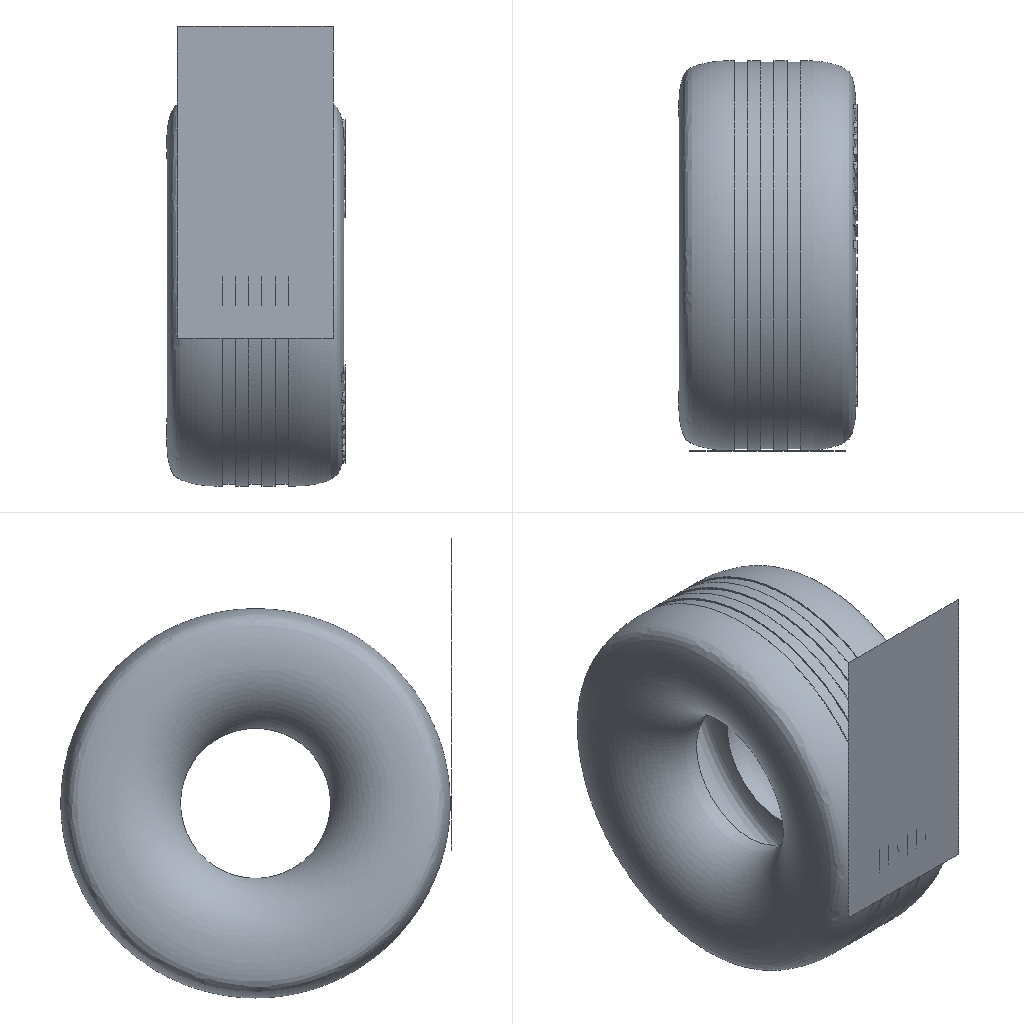Simulation study | abaqus
Set-up summary:
category,name,step,type,value,unit,region
solver,abaqus
solver,version,,,Abaqus/Explicit 2020
units,not stated in the deck,,not stated
analysis,deck,,transient,transient
load_step,Step-1,Step-1,transient
load_step,requested,,,1
mesh,nodes,,,158622
mesh,elements,,,81941
element_type,S4,,shell,5000
element_type,C3D10M,,solid,76941
load,load commands in deck,,count,3
bc,support commands in deck,,count,6
material,STEEL,,in results
material,XIANGJIAO,,in results
check,setup vs results,,match,"per instance, exact: element labels, types and connectivity; labels of the nodes the elements use; coordinates not compared"
Abaqus input file, long lists of numbers shortened:
*Heading
** Job name: Job-2 Model name: Model-2
** Generated by: Abaqus/CAE 2020
*Preprint, echo=NO, model=NO, history=NO, contact=NO
**
** PARTS
**
*Part, name=another-2
*Node
      1,       -273.5,           0.,         465.
      2,       -273.5,           0.,         485.
** (153469 more lines like these left out)
*Element, type=C3D10M
    1,  25421,    405,  19679,    406,  25558,  25557,  25556,  25560,  25559,  25561
    2,  25421,    233,    406,    220,  25563,  25562,  25560,  25565,  25564,  25566
** (76939 more lines like these left out)
*Nset, nset=Set-3, generate
      1,  153471,       1
*Elset, elset=Set-3, generate
     1,  76941,      1
** Section: xiangjiao
*Solid Section, elset=Set-3, material=xiangjiao
,
*End Part
**
*Part, name=road
*Node
      1,         290.,         915.,           0.
      2,         280.,         915.,           0.
** (5149 more lines like these left out)
*Element, type=S4
   1,    1,    2,   53,   52
   2,    2,    3,   54,   53
** (4998 more lines like these left out)
*Nset, nset=Set-1, generate
    1,  5151,     1
*Elset, elset=Set-1, generate
    1,  5000,     1
** Section: Section-1
*Shell Section, elset=Set-1, material=steel
10., 5
*End Part
**
**
** ASSEMBLY
**
*Assembly, name=Assembly
**
*Instance, name=road-1, part=road
        -40.,       -626.5,         -65.
        -40.,       -626.5,         -65., -39.,       -626.5,         -65., 90.
*End Instance
**
*Instance, name=another-2-1, part=another-2
*End Instance
**
*Node
      1,           0.,           0.,           0.
*Node
      2,         250.,       -626.5,         350.
*Nset, nset=Set-2, instance=road-1, generate
    1,  5151,     1
*Elset, elset=Set-2, instance=road-1, generate
    1,  5000,     1
*Nset, nset=Set-3
 1,
*Nset, nset=Set-5
 1,
*Nset, nset=Set-6
 1,
*Nset, nset=Set-7
 1,
*Nset, nset=Set-8
 1,
*Nset, nset=Set-9
 1,
*Nset, nset=Set-10
 1,
*Nset, nset=Set-13
 2,
*Nset, nset=Set-14
 2,
*Nset, nset=Set-15
 2,
*Nset, nset=Set-16
 1,
*Nset, nset=b_Set-11, instance=road-1, generate
    1,  5151,     1
*Elset, elset=b_Set-11, instance=road-1, generate
    1,  5000,     1
*Nset, nset=m_Set-1
 1,
*Nset, nset=_PickedSet569, internal
 2,
*Elset, elset=_m_Surf-6_S3, internal, instance=another-2-1
     2,     4,    11,    12,    21,    25,    27,    28,    33,    35,    36,    39,    44,    46,    52,    57
    63,    64,    68,    74,    80,    82,    95,   101,   110,   111,   113,   115,   117,   119,   125,   132
** (1293 more lines like these left out)
*Elset, elset=_m_Surf-6_S2, internal, instance=another-2-1
    13,    17,    24,    48,    76,    90,    91,   114,   130,   157,   162,   167,   189,   201,   203,   218
   219,   221,   223,   227,   236,   240,   244,   250,   253,   258,   260,   262,   264,   283,   286,   301
** (696 more lines like these left out)
*Elset, elset=_m_Surf-6_S4, internal, instance=another-2-1
    13,    17,    24,    72,    76,    90,    91,   127,   131,   138,   143,   144,   148,   149,   177,   182
   187,   200,   205,   209,   228,   229,   235,   239,   241,   249,   270,   287,   289,   315,   317,   340
** (553 more lines like these left out)
*Elset, elset=_m_Surf-6_S1, internal, instance=another-2-1
    77,    81,   102,   137,   142,   145,   147,   152,   163,   171,   176,   179,   183,   184,   188,   191
   194,   196,   199,   204,   213,   222,   254,   261,   292,   295,   298,   306,   312,   325,   327,   331
** (628 more lines like these left out)
*Surface, type=ELEMENT, name=m_Surf-6
_m_Surf-6_S3, S3
_m_Surf-6_S2, S2
_m_Surf-6_S4, S4
_m_Surf-6_S1, S1
*Elset, elset=_s_Surf-2_SNEG, internal, instance=road-1, generate
    1,  5000,     1
*Surface, type=ELEMENT, name=s_Surf-2
_s_Surf-2_SNEG, SNEG
*Elset, elset=_s_Surf-7_S2, internal, instance=another-2-1
   283,   778,   861,   891,  1202,  2571,  3390,  3572,  3582, 12767, 13246, 13428, 13452, 13654, 13655, 13845
 14168, 14374, 14473, 14524, 14556, 14585, 14654, 14658, 14901, 15060, 15256, 16243, 16332, 16818, 16869, 16954
** (48 more lines like these left out)
*Elset, elset=_s_Surf-7_S4, internal, instance=another-2-1
   534,  2030,  2716,  2979,  3068,  3096,  3405,  4405,  4516,  4563,  4617,  4650,  4711,  4880,  4964,  5366
  6105,  6179,  6937,  7172,  7302,  7446,  7558,  7648,  7711,  8438,  8761,  8846,  8929,  9299,  9464,  9589
** (42 more lines like these left out)
*Elset, elset=_s_Surf-7_S1, internal, instance=another-2-1
   147,  3780,  8101, 13221, 13303, 13883, 13888, 14132, 14412, 14921, 15604, 16206, 16210, 16278, 16845, 16964
 16975, 16991, 17238, 17275, 17350, 17860, 18733, 18770, 19022, 19134, 19143, 19535, 19597, 19622, 19631, 20059
** (38 more lines like these left out)
*Elset, elset=_s_Surf-7_S3, internal, instance=another-2-1
  3700,  8895,  9283,  9724, 10450, 12013, 12635, 12756, 12771, 12774, 12786, 12808, 12819, 12862, 12867, 12873
 12899, 12956, 12958, 13048, 13059, 13120, 13146, 13269, 13272, 13330, 13347, 13350, 13362, 13403, 13407, 13453
** (250 more lines like these left out)
*Surface, type=ELEMENT, name=s_Surf-7
_s_Surf-7_S2, S2
_s_Surf-7_S4, S4
_s_Surf-7_S1, S1
_s_Surf-7_S3, S3
*Elset, elset=_s_Surf-8_S1, internal, instance=another-2-1
   183,   602,   880,  1021,  1075,  1262,  1336,  1680,  1805,  1959,  1971,  2449,  2454,  2666,  2884,  2893
  3035,  3055,  3091,  3385,  3681,  3705,  3766,  3799,  3957,  4087,  4195,  4225,  4789,  4989,  5059,  5207
** (25 more lines like these left out)
*Elset, elset=_s_Surf-8_S2, internal, instance=another-2-1
   223,   310,   402,   647,   824,  2323,  2381,  2720,  3745,  3875,  4029,  4113,  4167,  5371,  5416,  5515
  6377,  7873,  8407,  8416,  8421,  8429,  8435,  8436,  8441,  8454,  8457,  8472,  8477,  8489,  8491,  8496
** (27 more lines like these left out)
*Elset, elset=_s_Surf-8_S4, internal, instance=another-2-1
   182,   351,   461,   471,   592,   640,   648,   654,   798,   810,   834,   986,  1061,  1207,  1269,  1474
  1634,  1707,  1708,  1927,  1976,  1986,  2055,  2143,  2235,  2291,  2459,  2586,  2791,  2992,  3083,  3110
** (28 more lines like these left out)
*Elset, elset=_s_Surf-8_S3, internal, instance=another-2-1
   132,   133,   134,   140,   146,   159,   160,   178,   180,   195,   202,   210,   212,   214,   216,   226
   230,   231,   247,   255,   256,   257,   267,   268,   271,   274,   281,   284,   302,   303,   304,   309
** (366 more lines like these left out)
*Surface, type=ELEMENT, name=s_Surf-8
_s_Surf-8_S1, S1
_s_Surf-8_S2, S2
_s_Surf-8_S4, S4
_s_Surf-8_S3, S3
*Elset, elset=_s_Surf-9_S2, internal, instance=another-2-1
   283,   778,   861,   891,  1202,  2571,  3390,  3572,  3582, 12767, 13246, 13428, 13452, 13654, 13655, 13845
 14168, 14374, 14473, 14524, 14556, 14585, 14654, 14658, 14901, 15060, 15256, 16243, 16332, 16818, 16869, 16954
** (48 more lines like these left out)
*Elset, elset=_s_Surf-9_S4, internal, instance=another-2-1
   534,  2030,  2716,  2979,  3068,  3096,  3405,  4405,  4516,  4563,  4617,  4650,  4711,  4880,  4964,  5366
  6105,  6179,  6937,  7172,  7302,  7446,  7558,  7648,  7711,  8438,  8761,  8846,  8929,  9299,  9464,  9589
** (42 more lines like these left out)
*Elset, elset=_s_Surf-9_S1, internal, instance=another-2-1
   147,  3780,  8101, 13221, 13303, 13883, 13888, 14132, 14412, 14921, 15604, 16206, 16210, 16278, 16845, 16964
 16975, 16991, 17238, 17275, 17350, 17860, 18733, 18770, 19022, 19134, 19143, 19535, 19597, 19622, 19631, 20059
** (38 more lines like these left out)
*Elset, elset=_s_Surf-9_S3, internal, instance=another-2-1
  3700,  8895,  9283,  9724, 10450, 12013, 12635, 12756, 12771, 12774, 12786, 12808, 12819, 12862, 12867, 12873
 12899, 12956, 12958, 13048, 13059, 13120, 13146, 13269, 13272, 13330, 13347, 13350, 13362, 13403, 13407, 13453
** (250 more lines like these left out)
*Surface, type=ELEMENT, name=s_Surf-9
_s_Surf-9_S2, S2
_s_Surf-9_S4, S4
_s_Surf-9_S1, S1
_s_Surf-9_S3, S3
*Elset, elset=_s_Surf-10_S3, internal, instance=another-2-1
    46,    52,    57,    63,    64,    68,   125,   156,   215,   332,   408,   440,   445,   490,   491,   626
   652,   655,   664,   684,   739,   787,   811,   876,   944,  1031,  1039,  1057,  1183,  1197,  1496,  1561
** (90 more lines like these left out)
*Elset, elset=_s_Surf-10_S2, internal, instance=another-2-1
    48,   130,   157,   162,   167,   189,   201,   203,   218,   219,   221,   227,   236,   240,   244,   250
   253,   258,   262,   264,   286,   301,   305,   307,   311,   314,   321,   323,   330,   334,   335,   337
** (416 more lines like these left out)
*Elset, elset=_s_Surf-10_S4, internal, instance=another-2-1
    72,   127,   131,   138,   143,   144,   148,   149,   177,   187,   200,   205,   209,   228,   229,   235
   239,   241,   249,   270,   287,   289,   315,   317,   348,   366,   376,   387,   420,   435,   441,   459
** (273 more lines like these left out)
*Elset, elset=_s_Surf-10_S1, internal, instance=another-2-1
    81,   137,   142,   145,   152,   163,   171,   176,   179,   184,   188,   191,   194,   196,   199,   204
   213,   222,   254,   261,   292,   295,   298,   306,   312,   325,   327,   331,   339,   341,   353,   364
** (368 more lines like these left out)
*Surface, type=ELEMENT, name=s_Surf-10
_s_Surf-10_S3, S3
_s_Surf-10_S2, S2
_s_Surf-10_S4, S4
_s_Surf-10_S1, S1
*Elset, elset=_s_Surf-11_S3, internal, instance=another-2-1
    46,    52,    57,    63,    64,    68,   125,   156,   215,   332,   408,   440,   445,   490,   491,   626
   652,   655,   664,   684,   739,   787,   811,   876,   944,  1031,  1039,  1057,  1183,  1197,  1496,  1561
** (90 more lines like these left out)
*Elset, elset=_s_Surf-11_S2, internal, instance=another-2-1
    48,   130,   157,   162,   167,   189,   201,   203,   218,   219,   221,   227,   236,   240,   244,   250
   253,   258,   262,   264,   286,   301,   305,   307,   311,   314,   321,   323,   330,   334,   335,   337
** (416 more lines like these left out)
*Elset, elset=_s_Surf-11_S4, internal, instance=another-2-1
    72,   127,   131,   138,   143,   144,   148,   149,   177,   187,   200,   205,   209,   228,   229,   235
   239,   241,   249,   270,   287,   289,   315,   317,   348,   366,   376,   387,   420,   435,   441,   459
** (273 more lines like these left out)
*Elset, elset=_s_Surf-11_S1, internal, instance=another-2-1
    81,   137,   142,   145,   152,   163,   171,   176,   179,   184,   188,   191,   194,   196,   199,   204
   213,   222,   254,   261,   292,   295,   298,   306,   312,   325,   327,   331,   339,   341,   353,   364
** (368 more lines like these left out)
*Surface, type=ELEMENT, name=s_Surf-11
_s_Surf-11_S3, S3
_s_Surf-11_S2, S2
_s_Surf-11_S4, S4
_s_Surf-11_S1, S1
*Elset, elset=_s_Surf-12_S1, internal, instance=another-2-1
  8410,  8474,  8493,  8543,  8557,  8567,  8624,  8628,  8662,  8678,  8684,  8712,  8715,  8722,  8723,  8732
  8738,  8745,  8758,  8760,  8762,  8764,  8772,  8778,  8783,  8789,  8792,  8793,  8863,  8890,  8898,  8913
** (11 more lines like these left out)
*Elset, elset=_s_Surf-12_S2, internal, instance=another-2-1
  3875,  8407,  8421,  8429,  8435,  8436,  8441,  8454,  8457,  8472,  8477,  8489,  8491,  8496,  8500,  8509
  8521,  8522,  8528,  8562,  8563,  8574,  8581,  8593,  8639,  8664,  8669,  8677,  8692,  8699,  8703,  8727
** (13 more lines like these left out)
*Elset, elset=_s_Surf-12_S4, internal, instance=another-2-1
  8443,  8448,  8461,  8490,  8510,  8513,  8538,  8572,  8582,  8584,  8595,  8603,  8616,  8623,  8629,  8634
  8641,  8649,  8655,  8672,  8690,  8701,  8710,  8731,  8750,  8787,  8825,  8840,  8861,  8880,  8966,  8987
** (7 more lines like these left out)
*Elset, elset=_s_Surf-12_S3, internal, instance=another-2-1
  8402,  8517,  8597,  8807,  8869,  8924,  9017, 12719, 13188, 13313, 14043, 17672, 20150, 22182, 24037, 25288
 25334, 25508, 25831, 26030, 27076, 27959, 28127, 28290, 33836, 34574, 71737
*Surface, type=ELEMENT, name=s_Surf-12
_s_Surf-12_S1, S1
_s_Surf-12_S2, S2
_s_Surf-12_S4, S4
_s_Surf-12_S3, S3
** Constraint: Constraint-1
*Coupling, constraint name=Constraint-1, ref node=m_Set-1, surface=s_Surf-12
*Kinematic
** Constraint: Constraint-2
*Rigid Body, ref node=_PickedSet569, elset=b_Set-11, position=CENTER OF MASS
*End Assembly
*Amplitude, name=Amp-1
             0.,              0.,            0.01,              1.
**
** MATERIALS
**
*Material, name=steel
*Density
 7.89e-09,
*Elastic
210000., 0.3
*Plastic
300.,0.
*Material, name=xiangjiao
*Density
 1.1e-09,
*Elastic
10000., 0.35
**
** INTERACTION PROPERTIES
**
*Surface Interaction, name=IntProp-1
*Friction
 0.4,
*Surface Behavior, pressure-overclosure=HARD
** ----------------------------------------------------------------
**
** STEP: Step-1
**
*Step, name=Step-1, nlgeom=YES
*Dynamic, Explicit
, 0.01
*Bulk Viscosity
0.06, 1.2
**
** BOUNDARY CONDITIONS
**
** Name: BC-1 Type: 对称/反对称/完全固定
*Boundary
Set-13, ENCASTRE
** Name: BC-3 Type: 速度/角速度
*Boundary, type=VELOCITY
Set-9, 1, 1
Set-9, 2, 2
Set-9, 4, 4, 1070.
Set-9, 5, 5
Set-9, 6, 6
**
** LOADS
**
** Name: Load-3   Type: Concentrated force
*Cload
Set-16, 2, -5000.
** Name: Load-4   Type: Gravity
*Dload
, GRAV, 9800., 0., -1., 0.
**
** INTERACTIONS
**
** Interaction: Int-2
*Contact Pair, interaction=IntProp-1, mechanical constraint=KINEMATIC, cpset=Int-2
s_Surf-2, m_Surf-6
**
** OUTPUT REQUESTS
**
*Restart, write, number interval=1, time marks=NO
**
** FIELD OUTPUT: F-Output-1
**
*Output, field, number interval=100
*Node Output
A, RF, RM, U, UR, V
*Element Output, directions=YES
E, LE, MISES, PE, PEEQ, S
*Contact Output
CFORCE, CSTRESS
**
** HISTORY OUTPUT: H-Output-1
**
*Output, history, variable=PRESELECT
*End Step
Results summary:
result,step,Step-1,partial,increments=4407 time=7.356984575569112e-05/0.01
result,analysis,,,transient
result,last_loadstep,,,1
result,primary field,,,"U, UR"
result,reaction total,,FX,-0.000752,model units
result,reaction total,,FY,5027.537,model units
result,reaction total,,FZ,0.0,model units